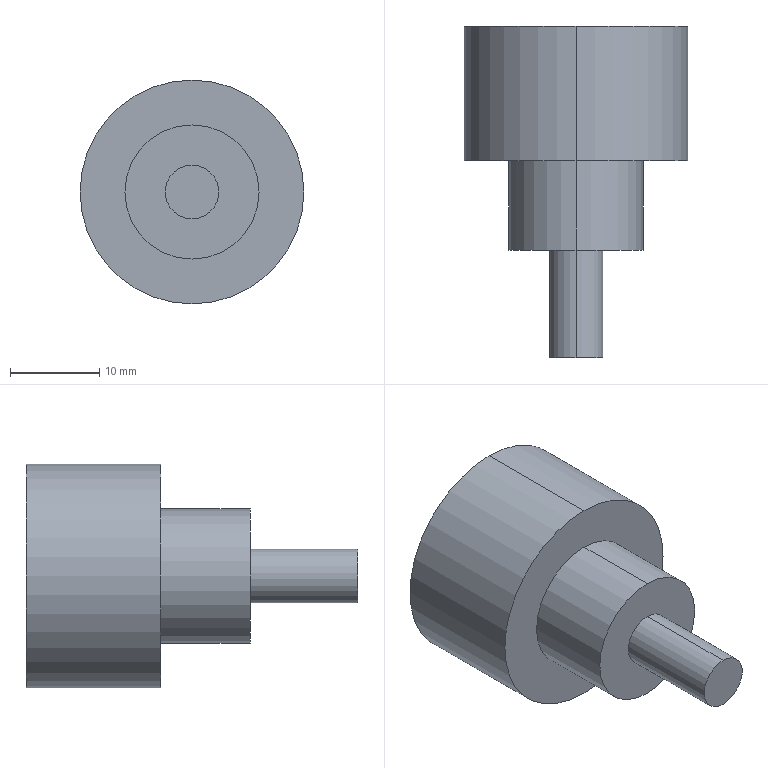Part | SolidWorks | features ICE 3, Extrusion 1 | 1 solid | 17 faces | box 25 x 37 x 25 mm | volume 7911 mm3 | plane 11 | cylinder 6 | commonest cylinder face diameters 6 x2 15 x2 25 x2
STEP:
#1=CARTESIAN_POINT('',(0.,37.,12.5));
#2=VERTEX_POINT('',#1);
#3=CARTESIAN_POINT('',(0.,37.,-12.5));
#4=VERTEX_POINT('',#3);
#5=CARTESIAN_POINT('',(0.,37.,0.));
#6=DIRECTION('',(0.,1.,0.));
#7=DIRECTION('',(0.,0.,1.));
#8=AXIS2_PLACEMENT_3D('',#5,#6,#7);
#9=CIRCLE('',#8,12.5);
#10=EDGE_CURVE('',#2,#4,#9,.T.);
#11=ORIENTED_EDGE('',*,*,#10,.F.);
#12=CARTESIAN_POINT('',(0.,22.,12.5));
#13=VERTEX_POINT('',#12);
#14=CARTESIAN_POINT('',(0.,37.,12.5));
#15=DIRECTION('',(0.,-1.,0.));
#16=VECTOR('',#15,1000.);
#17=LINE('',#14,#16);
#18=EDGE_CURVE('',#2,#13,#17,.T.);
#19=ORIENTED_EDGE('',*,*,#18,.T.);
#20=CARTESIAN_POINT('',(0.,22.,-12.5));
#21=VERTEX_POINT('',#20);
#22=CARTESIAN_POINT('',(0.,22.,0.));
#23=DIRECTION('',(0.,1.,0.));
#24=DIRECTION('',(0.,0.,1.));
#25=AXIS2_PLACEMENT_3D('',#22,#23,#24);
#26=CIRCLE('',#25,12.5);
#27=EDGE_CURVE('',#13,#21,#26,.T.);
#28=ORIENTED_EDGE('',*,*,#27,.T.);
#29=CARTESIAN_POINT('',(0.,37.,-12.5));
#30=DIRECTION('',(0.,-1.,0.));
#31=VECTOR('',#30,1000.);
#32=LINE('',#29,#31);
#33=EDGE_CURVE('',#4,#21,#32,.T.);
#34=ORIENTED_EDGE('',*,*,#33,.F.);
#35=EDGE_LOOP('',(#11,#19,#28,#34));
#36=FACE_OUTER_BOUND('',#35,.T.);
#37=CARTESIAN_POINT('',(0.,37.,0.));
#38=DIRECTION('',(0.,-1.,0.));
#39=DIRECTION('',(0.,0.,-1.));
#40=AXIS2_PLACEMENT_3D('',#37,#38,#39);
#41=CYLINDRICAL_SURFACE('',#40,12.5);
#42=ADVANCED_FACE('',(#36),#41,.T.);
#43=CARTESIAN_POINT('',(0.,22.,7.5));
#44=VERTEX_POINT('',#43);
#45=CARTESIAN_POINT('',(0.,22.,-7.5));
#46=VERTEX_POINT('',#45);
#47=CARTESIAN_POINT('',(0.,22.,0.));
#48=DIRECTION('',(0.,1.,0.));
#49=DIRECTION('',(0.,0.,1.));
#50=AXIS2_PLACEMENT_3D('',#47,#48,#49);
#51=CIRCLE('',#50,7.5);
#52=EDGE_CURVE('',#44,#46,#51,.T.);
#53=ORIENTED_EDGE('',*,*,#52,.F.);
#54=CARTESIAN_POINT('',(0.,12.,7.5));
#55=VERTEX_POINT('',#54);
#56=CARTESIAN_POINT('',(0.,22.,7.5));
#57=DIRECTION('',(0.,-1.,0.));
#58=VECTOR('',#57,1000.);
#59=LINE('',#56,#58);
#60=EDGE_CURVE('',#44,#55,#59,.T.);
#61=ORIENTED_EDGE('',*,*,#60,.T.);
#62=CARTESIAN_POINT('',(0.,12.,-7.5));
#63=VERTEX_POINT('',#62);
#64=CARTESIAN_POINT('',(0.,12.,0.));
#65=DIRECTION('',(0.,1.,0.));
#66=DIRECTION('',(0.,0.,1.));
#67=AXIS2_PLACEMENT_3D('',#64,#65,#66);
#68=CIRCLE('',#67,7.5);
#69=EDGE_CURVE('',#55,#63,#68,.T.);
#70=ORIENTED_EDGE('',*,*,#69,.T.);
#71=CARTESIAN_POINT('',(0.,22.,-7.5));
#72=DIRECTION('',(0.,-1.,0.));
#73=VECTOR('',#72,1000.);
#74=LINE('',#71,#73);
#75=EDGE_CURVE('',#46,#63,#74,.T.);
#76=ORIENTED_EDGE('',*,*,#75,.F.);
#77=EDGE_LOOP('',(#53,#61,#70,#76));
#78=FACE_OUTER_BOUND('',#77,.T.);
#79=CARTESIAN_POINT('',(0.,22.,0.));
#80=DIRECTION('',(0.,-1.,0.));
#81=DIRECTION('',(0.,0.,-1.));
#82=AXIS2_PLACEMENT_3D('',#79,#80,#81);
#83=CYLINDRICAL_SURFACE('',#82,7.5);
#84=ADVANCED_FACE('',(#78),#83,.T.);
#85=CARTESIAN_POINT('',(0.,12.,3.));
#86=VERTEX_POINT('',#85);
#87=CARTESIAN_POINT('',(0.,12.,-3.));
#88=VERTEX_POINT('',#87);
#89=CARTESIAN_POINT('',(0.,12.,0.));
#90=DIRECTION('',(0.,1.,0.));
#91=DIRECTION('',(0.,0.,1.));
#92=AXIS2_PLACEMENT_3D('',#89,#90,#91);
#93=CIRCLE('',#92,3.);
#94=EDGE_CURVE('',#86,#88,#93,.T.);
#95=ORIENTED_EDGE('',*,*,#94,.F.);
#96=CARTESIAN_POINT('',(0.,0.,3.));
#97=VERTEX_POINT('',#96);
#98=CARTESIAN_POINT('',(0.,12.,3.));
#99=DIRECTION('',(0.,-1.,0.));
#100=VECTOR('',#99,1000.);
#101=LINE('',#98,#100);
#102=EDGE_CURVE('',#86,#97,#101,.T.);
#103=ORIENTED_EDGE('',*,*,#102,.T.);
#104=CARTESIAN_POINT('',(0.,0.,-3.));
#105=VERTEX_POINT('',#104);
#106=CARTESIAN_POINT('',(0.,0.,0.));
#107=DIRECTION('',(0.,1.,0.));
#108=DIRECTION('',(0.,0.,1.));
#109=AXIS2_PLACEMENT_3D('',#106,#107,#108);
#110=CIRCLE('',#109,3.);
#111=EDGE_CURVE('',#97,#105,#110,.T.);
#112=ORIENTED_EDGE('',*,*,#111,.T.);
#113=CARTESIAN_POINT('',(0.,12.,-3.));
#114=DIRECTION('',(0.,-1.,0.));
#115=VECTOR('',#114,1000.);
#116=LINE('',#113,#115);
#117=EDGE_CURVE('',#88,#105,#116,.T.);
#118=ORIENTED_EDGE('',*,*,#117,.F.);
#119=EDGE_LOOP('',(#95,#103,#112,#118));
#120=FACE_OUTER_BOUND('',#119,.T.);
#121=CARTESIAN_POINT('',(0.,12.,0.));
#122=DIRECTION('',(0.,-1.,0.));
#123=DIRECTION('',(0.,0.,-1.));
#124=AXIS2_PLACEMENT_3D('',#121,#122,#123);
#125=CYLINDRICAL_SURFACE('',#124,3.);
#126=ADVANCED_FACE('',(#120),#125,.T.);
#127=ORIENTED_EDGE('',*,*,#102,.F.);
#128=CARTESIAN_POINT('',(0.,12.,0.));
#129=DIRECTION('',(0.,1.,0.));
#130=DIRECTION('',(0.,0.,1.));
#131=AXIS2_PLACEMENT_3D('',#128,#129,#130);
#132=CIRCLE('',#131,3.);
#133=EDGE_CURVE('',#88,#86,#132,.T.);
#134=ORIENTED_EDGE('',*,*,#133,.F.);
#135=ORIENTED_EDGE('',*,*,#117,.T.);
#136=CARTESIAN_POINT('',(0.,0.,0.));
#137=DIRECTION('',(0.,1.,0.));
#138=DIRECTION('',(0.,0.,1.));
#139=AXIS2_PLACEMENT_3D('',#136,#137,#138);
#140=CIRCLE('',#139,3.);
#141=EDGE_CURVE('',#105,#97,#140,.T.);
#142=ORIENTED_EDGE('',*,*,#141,.T.);
#143=EDGE_LOOP('',(#127,#134,#135,#142));
#144=FACE_OUTER_BOUND('',#143,.T.);
#145=CARTESIAN_POINT('',(0.,12.,0.));
#146=DIRECTION('',(0.,-1.,0.));
#147=DIRECTION('',(0.,0.,-1.));
#148=AXIS2_PLACEMENT_3D('',#145,#146,#147);
#149=CYLINDRICAL_SURFACE('',#148,3.);
#150=ADVANCED_FACE('',(#144),#149,.T.);
#151=ORIENTED_EDGE('',*,*,#141,.F.);
#152=ORIENTED_EDGE('',*,*,#111,.F.);
#153=EDGE_LOOP('',(#151,#152));
#154=FACE_OUTER_BOUND('',#153,.T.);
#155=CARTESIAN_POINT('',(0.,0.,0.));
#156=DIRECTION('',(0.,1.,0.));
#157=DIRECTION('',(0.,0.,1.));
#158=AXIS2_PLACEMENT_3D('',#155,#156,#157);
#159=PLANE('',#158);
#160=ADVANCED_FACE('',(#154),#159,.F.);
#161=ORIENTED_EDGE('',*,*,#60,.F.);
#162=CARTESIAN_POINT('',(0.,22.,0.));
#163=DIRECTION('',(0.,1.,0.));
#164=DIRECTION('',(0.,0.,1.));
#165=AXIS2_PLACEMENT_3D('',#162,#163,#164);
#166=CIRCLE('',#165,7.5);
#167=EDGE_CURVE('',#46,#44,#166,.T.);
#168=ORIENTED_EDGE('',*,*,#167,.F.);
#169=ORIENTED_EDGE('',*,*,#75,.T.);
#170=CARTESIAN_POINT('',(0.,12.,0.));
#171=DIRECTION('',(0.,1.,0.));
#172=DIRECTION('',(0.,0.,1.));
#173=AXIS2_PLACEMENT_3D('',#170,#171,#172);
#174=CIRCLE('',#173,7.5);
#175=EDGE_CURVE('',#63,#55,#174,.T.);
#176=ORIENTED_EDGE('',*,*,#175,.T.);
#177=EDGE_LOOP('',(#161,#168,#169,#176));
#178=FACE_OUTER_BOUND('',#177,.T.);
#179=CARTESIAN_POINT('',(0.,22.,0.));
#180=DIRECTION('',(0.,-1.,0.));
#181=DIRECTION('',(0.,0.,-1.));
#182=AXIS2_PLACEMENT_3D('',#179,#180,#181);
#183=CYLINDRICAL_SURFACE('',#182,7.5);
#184=ADVANCED_FACE('',(#178),#183,.T.);
#185=ORIENTED_EDGE('',*,*,#133,.T.);
#186=ORIENTED_EDGE('',*,*,#94,.T.);
#187=EDGE_LOOP('',(#185,#186));
#188=FACE_BOUND('',#187,.T.);
#189=ORIENTED_EDGE('',*,*,#175,.F.);
#190=ORIENTED_EDGE('',*,*,#69,.F.);
#191=EDGE_LOOP('',(#189,#190));
#192=FACE_OUTER_BOUND('',#191,.T.);
#193=CARTESIAN_POINT('',(0.,12.,0.));
#194=DIRECTION('',(0.,1.,0.));
#195=DIRECTION('',(0.,0.,1.));
#196=AXIS2_PLACEMENT_3D('',#193,#194,#195);
#197=PLANE('',#196);
#198=ADVANCED_FACE('',(#188,#192),#197,.F.);
#199=ORIENTED_EDGE('',*,*,#18,.F.);
#200=CARTESIAN_POINT('',(0.,37.,0.));
#201=DIRECTION('',(0.,1.,0.));
#202=DIRECTION('',(0.,0.,1.));
#203=AXIS2_PLACEMENT_3D('',#200,#201,#202);
#204=CIRCLE('',#203,12.5);
#205=EDGE_CURVE('',#4,#2,#204,.T.);
#206=ORIENTED_EDGE('',*,*,#205,.F.);
#207=ORIENTED_EDGE('',*,*,#33,.T.);
#208=CARTESIAN_POINT('',(0.,22.,0.));
#209=DIRECTION('',(0.,1.,0.));
#210=DIRECTION('',(0.,0.,1.));
#211=AXIS2_PLACEMENT_3D('',#208,#209,#210);
#212=CIRCLE('',#211,12.5);
#213=EDGE_CURVE('',#21,#13,#212,.T.);
#214=ORIENTED_EDGE('',*,*,#213,.T.);
#215=EDGE_LOOP('',(#199,#206,#207,#214));
#216=FACE_OUTER_BOUND('',#215,.T.);
#217=CARTESIAN_POINT('',(0.,37.,0.));
#218=DIRECTION('',(0.,-1.,0.));
#219=DIRECTION('',(0.,0.,-1.));
#220=AXIS2_PLACEMENT_3D('',#217,#218,#219);
#221=CYLINDRICAL_SURFACE('',#220,12.5);
#222=ADVANCED_FACE('',(#216),#221,.T.);
#223=CARTESIAN_POINT('',(7.5,37.,-4.33));
#224=VERTEX_POINT('',#223);
#225=CARTESIAN_POINT('',(0.,37.,-8.66));
#226=VERTEX_POINT('',#225);
#227=CARTESIAN_POINT('',(7.5,37.,-4.33));
#228=DIRECTION('',(-0.866,0.,-0.5));
#229=VECTOR('',#228,1000.);
#230=LINE('',#227,#229);
#231=EDGE_CURVE('',#224,#226,#230,.T.);
#232=ORIENTED_EDGE('',*,*,#231,.F.);
#233=CARTESIAN_POINT('',(7.5,37.,4.33));
#234=VERTEX_POINT('',#233);
#235=CARTESIAN_POINT('',(7.5,37.,4.33));
#236=DIRECTION('',(0.,0.,-1.));
#237=VECTOR('',#236,1000.);
#238=LINE('',#235,#237);
#239=EDGE_CURVE('',#234,#224,#238,.T.);
#240=ORIENTED_EDGE('',*,*,#239,.F.);
#241=CARTESIAN_POINT('',(0.,37.,8.66));
#242=VERTEX_POINT('',#241);
#243=CARTESIAN_POINT('',(0.,37.,8.66));
#244=DIRECTION('',(0.866,0.,-0.5));
#245=VECTOR('',#244,1000.);
#246=LINE('',#243,#245);
#247=EDGE_CURVE('',#242,#234,#246,.T.);
#248=ORIENTED_EDGE('',*,*,#247,.F.);
#249=CARTESIAN_POINT('',(-7.5,37.,4.33));
#250=VERTEX_POINT('',#249);
#251=CARTESIAN_POINT('',(-7.5,37.,4.33));
#252=DIRECTION('',(0.866,0.,0.5));
#253=VECTOR('',#252,1000.);
#254=LINE('',#251,#253);
#255=EDGE_CURVE('',#250,#242,#254,.T.);
#256=ORIENTED_EDGE('',*,*,#255,.F.);
#257=CARTESIAN_POINT('',(-7.5,37.,-4.33));
#258=VERTEX_POINT('',#257);
#259=CARTESIAN_POINT('',(-7.5,37.,-4.33));
#260=DIRECTION('',(0.,0.,1.));
#261=VECTOR('',#260,1000.);
#262=LINE('',#259,#261);
#263=EDGE_CURVE('',#258,#250,#262,.T.);
#264=ORIENTED_EDGE('',*,*,#263,.F.);
#265=CARTESIAN_POINT('',(0.,37.,-8.66));
#266=DIRECTION('',(-0.866,0.,0.5));
#267=VECTOR('',#266,1000.);
#268=LINE('',#265,#267);
#269=EDGE_CURVE('',#226,#258,#268,.T.);
#270=ORIENTED_EDGE('',*,*,#269,.F.);
#271=EDGE_LOOP('',(#232,#240,#248,#256,#264,#270));
#272=FACE_BOUND('',#271,.T.);
#273=ORIENTED_EDGE('',*,*,#205,.T.);
#274=ORIENTED_EDGE('',*,*,#10,.T.);
#275=EDGE_LOOP('',(#273,#274));
#276=FACE_OUTER_BOUND('',#275,.T.);
#277=CARTESIAN_POINT('',(0.,37.,0.));
#278=DIRECTION('',(0.,1.,0.));
#279=DIRECTION('',(0.,0.,1.));
#280=AXIS2_PLACEMENT_3D('',#277,#278,#279);
#281=PLANE('',#280);
#282=ADVANCED_FACE('',(#272,#276),#281,.T.);
#283=ORIENTED_EDGE('',*,*,#167,.T.);
#284=ORIENTED_EDGE('',*,*,#52,.T.);
#285=EDGE_LOOP('',(#283,#284));
#286=FACE_BOUND('',#285,.T.);
#287=ORIENTED_EDGE('',*,*,#213,.F.);
#288=ORIENTED_EDGE('',*,*,#27,.F.);
#289=EDGE_LOOP('',(#287,#288));
#290=FACE_OUTER_BOUND('',#289,.T.);
#291=CARTESIAN_POINT('',(0.,22.,0.));
#292=DIRECTION('',(0.,1.,0.));
#293=DIRECTION('',(0.,0.,1.));
#294=AXIS2_PLACEMENT_3D('',#291,#292,#293);
#295=PLANE('',#294);
#296=ADVANCED_FACE('',(#286,#290),#295,.F.);
#297=ORIENTED_EDGE('',*,*,#231,.T.);
#298=CARTESIAN_POINT('',(0.,29.,-8.66));
#299=VERTEX_POINT('',#298);
#300=CARTESIAN_POINT('',(0.,29.,-8.66));
#301=DIRECTION('',(0.,1.,0.));
#302=VECTOR('',#301,1000.);
#303=LINE('',#300,#302);
#304=EDGE_CURVE('',#299,#226,#303,.T.);
#305=ORIENTED_EDGE('',*,*,#304,.F.);
#306=CARTESIAN_POINT('',(7.5,29.,-4.33));
#307=VERTEX_POINT('',#306);
#308=CARTESIAN_POINT('',(7.5,29.,-4.33));
#309=DIRECTION('',(-0.866,0.,-0.5));
#310=VECTOR('',#309,1000.);
#311=LINE('',#308,#310);
#312=EDGE_CURVE('',#307,#299,#311,.T.);
#313=ORIENTED_EDGE('',*,*,#312,.F.);
#314=CARTESIAN_POINT('',(7.5,29.,-4.33));
#315=DIRECTION('',(0.,1.,0.));
#316=VECTOR('',#315,1000.);
#317=LINE('',#314,#316);
#318=EDGE_CURVE('',#307,#224,#317,.T.);
#319=ORIENTED_EDGE('',*,*,#318,.T.);
#320=EDGE_LOOP('',(#297,#305,#313,#319));
#321=FACE_OUTER_BOUND('',#320,.T.);
#322=CARTESIAN_POINT('',(7.5,29.,-4.33));
#323=DIRECTION('',(0.5,0.,-0.866));
#324=DIRECTION('',(-0.866,0.,-0.5));
#325=AXIS2_PLACEMENT_3D('',#322,#323,#324);
#326=PLANE('',#325);
#327=ADVANCED_FACE('',(#321),#326,.F.);
#328=ORIENTED_EDGE('',*,*,#239,.T.);
#329=ORIENTED_EDGE('',*,*,#318,.F.);
#330=CARTESIAN_POINT('',(7.5,29.,4.33));
#331=VERTEX_POINT('',#330);
#332=CARTESIAN_POINT('',(7.5,29.,4.33));
#333=DIRECTION('',(0.,0.,-1.));
#334=VECTOR('',#333,1000.);
#335=LINE('',#332,#334);
#336=EDGE_CURVE('',#331,#307,#335,.T.);
#337=ORIENTED_EDGE('',*,*,#336,.F.);
#338=CARTESIAN_POINT('',(7.5,29.,4.33));
#339=DIRECTION('',(0.,1.,0.));
#340=VECTOR('',#339,1000.);
#341=LINE('',#338,#340);
#342=EDGE_CURVE('',#331,#234,#341,.T.);
#343=ORIENTED_EDGE('',*,*,#342,.T.);
#344=EDGE_LOOP('',(#328,#329,#337,#343));
#345=FACE_OUTER_BOUND('',#344,.T.);
#346=CARTESIAN_POINT('',(7.5,29.,4.33));
#347=DIRECTION('',(1.,0.,0.));
#348=DIRECTION('',(0.,0.,-1.));
#349=AXIS2_PLACEMENT_3D('',#346,#347,#348);
#350=PLANE('',#349);
#351=ADVANCED_FACE('',(#345),#350,.F.);
#352=ORIENTED_EDGE('',*,*,#247,.T.);
#353=ORIENTED_EDGE('',*,*,#342,.F.);
#354=CARTESIAN_POINT('',(0.,29.,8.66));
#355=VERTEX_POINT('',#354);
#356=CARTESIAN_POINT('',(0.,29.,8.66));
#357=DIRECTION('',(0.866,0.,-0.5));
#358=VECTOR('',#357,1000.);
#359=LINE('',#356,#358);
#360=EDGE_CURVE('',#355,#331,#359,.T.);
#361=ORIENTED_EDGE('',*,*,#360,.F.);
#362=CARTESIAN_POINT('',(0.,29.,8.66));
#363=DIRECTION('',(0.,1.,0.));
#364=VECTOR('',#363,1000.);
#365=LINE('',#362,#364);
#366=EDGE_CURVE('',#355,#242,#365,.T.);
#367=ORIENTED_EDGE('',*,*,#366,.T.);
#368=EDGE_LOOP('',(#352,#353,#361,#367));
#369=FACE_OUTER_BOUND('',#368,.T.);
#370=CARTESIAN_POINT('',(0.,29.,8.66));
#371=DIRECTION('',(0.5,0.,0.866));
#372=DIRECTION('',(0.866,0.,-0.5));
#373=AXIS2_PLACEMENT_3D('',#370,#371,#372);
#374=PLANE('',#373);
#375=ADVANCED_FACE('',(#369),#374,.F.);
#376=ORIENTED_EDGE('',*,*,#255,.T.);
#377=ORIENTED_EDGE('',*,*,#366,.F.);
#378=CARTESIAN_POINT('',(-7.5,29.,4.33));
#379=VERTEX_POINT('',#378);
#380=CARTESIAN_POINT('',(-7.5,29.,4.33));
#381=DIRECTION('',(0.866,0.,0.5));
#382=VECTOR('',#381,1000.);
#383=LINE('',#380,#382);
#384=EDGE_CURVE('',#379,#355,#383,.T.);
#385=ORIENTED_EDGE('',*,*,#384,.F.);
#386=CARTESIAN_POINT('',(-7.5,29.,4.33));
#387=DIRECTION('',(0.,1.,0.));
#388=VECTOR('',#387,1000.);
#389=LINE('',#386,#388);
#390=EDGE_CURVE('',#379,#250,#389,.T.);
#391=ORIENTED_EDGE('',*,*,#390,.T.);
#392=EDGE_LOOP('',(#376,#377,#385,#391));
#393=FACE_OUTER_BOUND('',#392,.T.);
#394=CARTESIAN_POINT('',(-7.5,29.,4.33));
#395=DIRECTION('',(-0.5,0.,0.866));
#396=DIRECTION('',(0.866,0.,0.5));
#397=AXIS2_PLACEMENT_3D('',#394,#395,#396);
#398=PLANE('',#397);
#399=ADVANCED_FACE('',(#393),#398,.F.);
#400=ORIENTED_EDGE('',*,*,#263,.T.);
#401=ORIENTED_EDGE('',*,*,#390,.F.);
#402=CARTESIAN_POINT('',(-7.5,29.,-4.33));
#403=VERTEX_POINT('',#402);
#404=CARTESIAN_POINT('',(-7.5,29.,-4.33));
#405=DIRECTION('',(0.,0.,1.));
#406=VECTOR('',#405,1000.);
#407=LINE('',#404,#406);
#408=EDGE_CURVE('',#403,#379,#407,.T.);
#409=ORIENTED_EDGE('',*,*,#408,.F.);
#410=CARTESIAN_POINT('',(-7.5,29.,-4.33));
#411=DIRECTION('',(0.,1.,0.));
#412=VECTOR('',#411,1000.);
#413=LINE('',#410,#412);
#414=EDGE_CURVE('',#403,#258,#413,.T.);
#415=ORIENTED_EDGE('',*,*,#414,.T.);
#416=EDGE_LOOP('',(#400,#401,#409,#415));
#417=FACE_OUTER_BOUND('',#416,.T.);
#418=CARTESIAN_POINT('',(-7.5,29.,-4.33));
#419=DIRECTION('',(-1.,0.,0.));
#420=DIRECTION('',(0.,0.,1.));
#421=AXIS2_PLACEMENT_3D('',#418,#419,#420);
#422=PLANE('',#421);
#423=ADVANCED_FACE('',(#417),#422,.F.);
#424=ORIENTED_EDGE('',*,*,#269,.T.);
#425=ORIENTED_EDGE('',*,*,#414,.F.);
#426=CARTESIAN_POINT('',(0.,29.,-8.66));
#427=DIRECTION('',(-0.866,0.,0.5));
#428=VECTOR('',#427,1000.);
#429=LINE('',#426,#428);
#430=EDGE_CURVE('',#299,#403,#429,.T.);
#431=ORIENTED_EDGE('',*,*,#430,.F.);
#432=ORIENTED_EDGE('',*,*,#304,.T.);
#433=EDGE_LOOP('',(#424,#425,#431,#432));
#434=FACE_OUTER_BOUND('',#433,.T.);
#435=CARTESIAN_POINT('',(0.,29.,-8.66));
#436=DIRECTION('',(-0.5,0.,-0.866));
#437=DIRECTION('',(-0.866,0.,0.5));
#438=AXIS2_PLACEMENT_3D('',#435,#436,#437);
#439=PLANE('',#438);
#440=ADVANCED_FACE('',(#434),#439,.F.);
#441=ORIENTED_EDGE('',*,*,#312,.T.);
#442=ORIENTED_EDGE('',*,*,#430,.T.);
#443=ORIENTED_EDGE('',*,*,#408,.T.);
#444=ORIENTED_EDGE('',*,*,#384,.T.);
#445=ORIENTED_EDGE('',*,*,#360,.T.);
#446=ORIENTED_EDGE('',*,*,#336,.T.);
#447=EDGE_LOOP('',(#441,#442,#443,#444,#445,#446));
#448=FACE_OUTER_BOUND('',#447,.T.);
#449=CARTESIAN_POINT('',(0.,29.,0.));
#450=DIRECTION('',(0.,1.,0.));
#451=DIRECTION('',(0.,0.,1.));
#452=AXIS2_PLACEMENT_3D('',#449,#450,#451);
#453=PLANE('',#452);
#454=ADVANCED_FACE('',(#448),#453,.T.);
#455=CLOSED_SHELL('',(#42,#84,#126,#150,#160,#184,#198,#222,#282,#296,#327,#351,#375,#399,#423,#440,#454));
#456=MANIFOLD_SOLID_BREP('',#455);
#457=CARTESIAN_POINT('',(0.,0.,0.));
#458=DIRECTION('',(0.,0.,1.));
#459=DIRECTION('',(1.,0.,0.));
#460=AXIS2_PLACEMENT_3D('',#457,#458,#459);
#461=(LENGTH_UNIT()NAMED_UNIT(*)SI_UNIT(.MILLI.,.METRE.));
#462=UNCERTAINTY_MEASURE_WITH_UNIT(LENGTH_MEASURE(0.00001),#461,'','');
#463=(NAMED_UNIT(*)PLANE_ANGLE_UNIT()SI_UNIT($,.RADIAN.));
#464=(NAMED_UNIT(*)SI_UNIT($,.STERADIAN.)SOLID_ANGLE_UNIT());
#465=(GEOMETRIC_REPRESENTATION_CONTEXT(3)GLOBAL_UNCERTAINTY_ASSIGNED_CONTEXT((#462))GLOBAL_UNIT_ASSIGNED_CONTEXT((#461,#463,#464))REPRESENTATION_CONTEXT('',''));
#466=ADVANCED_BREP_SHAPE_REPRESENTATION('',(#456,#460),#465);